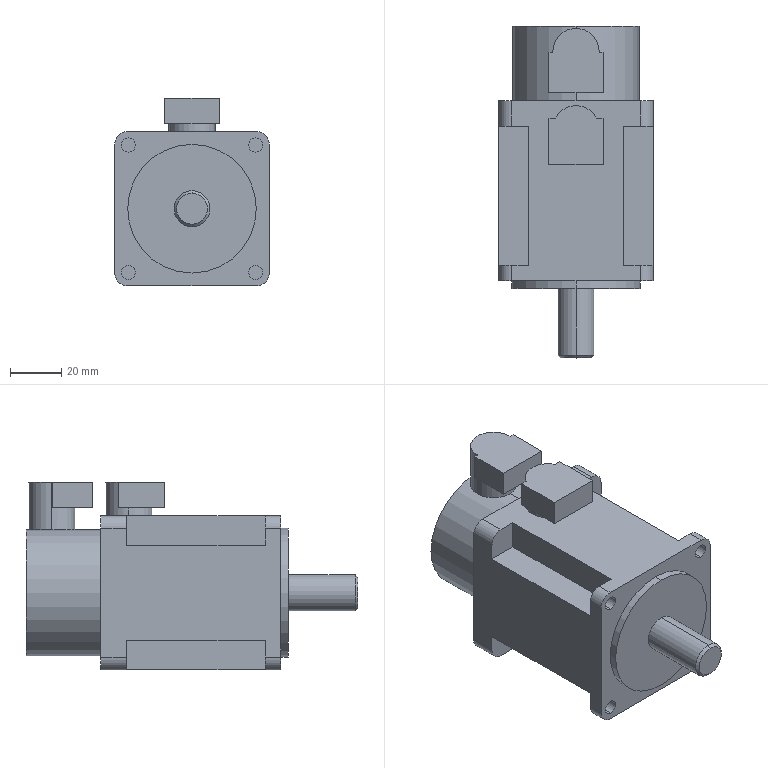Part | STEP file | SGMJV-04ADE6S (Yaskawa Servo 0.4KW) | 2 solids | 68 faces | box 60 x 129 x 73 mm | volume 298777 mm3 | plane 40 | cylinder 26 | cone 2 | commonest cylinder face diameters 5.5 x8 10 x8 18 x4 14 x2 49 x2 50 x2